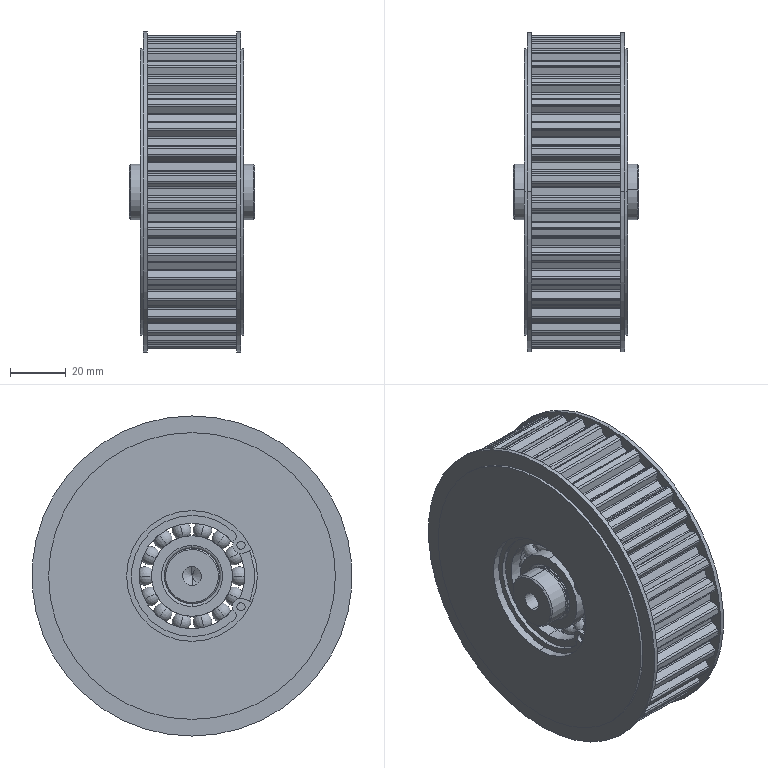Part | SolidWorks | 5 solids | 580 faces | box 45 x 115 x 115 mm | volume 326857 mm3 | cylinder 275 | plane 135 | torus 106 | sphere 56 | cone 8 | commonest cylinder face diameters 1.6 x86 1.2 x84 112.74 x36 20 x10 29 x8 38 x8